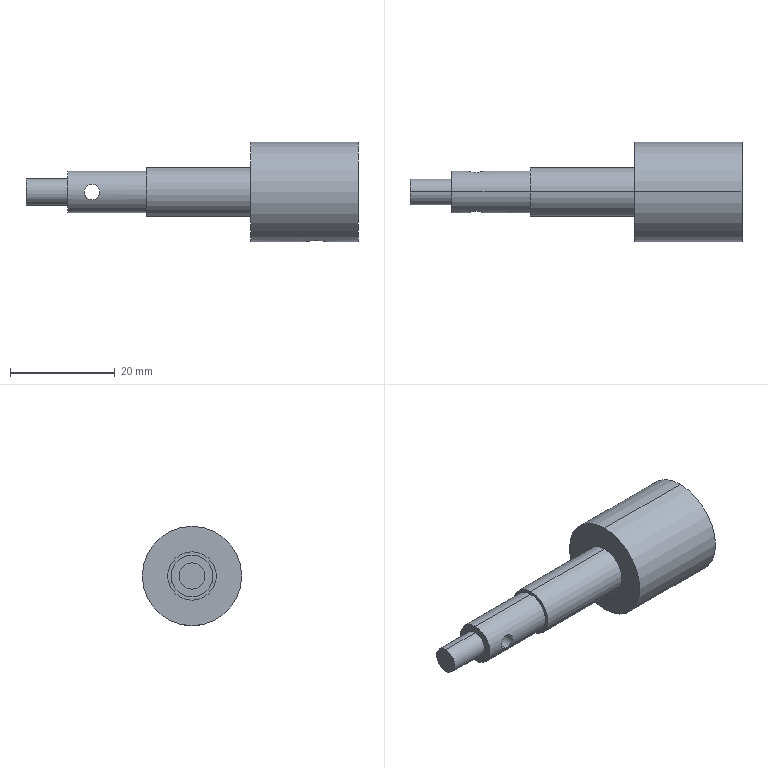Part | SolidWorks | features BaseBody 1 | 1 solid | 20 faces | box 63.5 x 19 x 19 mm | volume 6544 mm3 | cylinder 14 | plane 6 | commonest cylinder face diameters 3 x2 4 x2 5 x2 8 x2 9.26 x2 10 x2
STEP:
#1=CARTESIAN_POINT('',(-19.873,0.,-9.5));
#2=VERTEX_POINT('',#1);
#3=CARTESIAN_POINT('',(-15.873,0.,-9.5));
#4=VERTEX_POINT('',#3);
#5=CARTESIAN_POINT('',(-19.873,0.,-9.5));
#6=CARTESIAN_POINT('',(-19.873,-0.2614,-9.5));
#7=CARTESIAN_POINT('',(-19.82,-0.5253,-9.489));
#8=CARTESIAN_POINT('',(-19.67,-0.8864,-9.459));
#9=CARTESIAN_POINT('',(-19.608,-1.003,-9.448));
#10=CARTESIAN_POINT('',(-19.462,-1.221,-9.422));
#11=CARTESIAN_POINT('',(-19.38,-1.321,-9.408));
#12=CARTESIAN_POINT('',(-19.196,-1.506,-9.38));
#13=CARTESIAN_POINT('',(-19.093,-1.59,-9.366));
#14=CARTESIAN_POINT('',(-18.877,-1.735,-9.341));
#15=CARTESIAN_POINT('',(-18.762,-1.796,-9.329));
#16=CARTESIAN_POINT('',(-18.398,-1.948,-9.299));
#17=CARTESIAN_POINT('',(-18.138,-2.,-9.287));
#18=CARTESIAN_POINT('',(-17.742,-2.,-9.287));
#19=CARTESIAN_POINT('',(-17.612,-1.987,-9.29));
#20=CARTESIAN_POINT('',(-17.355,-1.936,-9.301));
#21=CARTESIAN_POINT('',(-17.228,-1.898,-9.309));
#22=CARTESIAN_POINT('',(-16.986,-1.797,-9.329));
#23=CARTESIAN_POINT('',(-16.871,-1.736,-9.34));
#24=CARTESIAN_POINT('',(-16.653,-1.591,-9.366));
#25=CARTESIAN_POINT('',(-16.551,-1.507,-9.38));
#26=CARTESIAN_POINT('',(-16.276,-1.231,-9.422));
#27=CARTESIAN_POINT('',(-16.126,-1.009,-9.449));
#28=CARTESIAN_POINT('',(-15.976,-0.6483,-9.479));
#29=CARTESIAN_POINT('',(-15.937,-0.5213,-9.487));
#30=CARTESIAN_POINT('',(-15.886,-0.2633,-9.497));
#31=CARTESIAN_POINT('',(-15.873,-0.1325,-9.5));
#32=CARTESIAN_POINT('',(-15.873,0.,-9.5));
#33=B_SPLINE_CURVE_WITH_KNOTS('',3,(#5,#6,#7,#8,#9,#10,#11,#12,#13,#14,#15,#16,#17,#18,#19,#20,#21,#22,#23,#24,#25,#26,#27,#28,#29,#30,#31,#32),.UNSPECIFIED.,.F.,.F.,(4,2,2,2,2,2,2,2,2,2,2,2,2,4),(0.00627,0.007054,0.007446,0.007838,0.00823,0.008621,0.009405,0.009797,0.01019,0.01058,0.01097,0.01176,0.01215,0.01254),.UNSPECIFIED.);
#34=EDGE_CURVE('',#2,#4,#33,.T.);
#35=ORIENTED_EDGE('',*,*,#34,.F.);
#36=CARTESIAN_POINT('',(-19.873,0.,-5.));
#37=VERTEX_POINT('',#36);
#38=CARTESIAN_POINT('',(-19.873,0.,-17.5));
#39=DIRECTION('',(0.,0.,1.));
#40=VECTOR('',#39,1000.);
#41=LINE('',#38,#40);
#42=EDGE_CURVE('',#2,#37,#41,.T.);
#43=ORIENTED_EDGE('',*,*,#42,.T.);
#44=CARTESIAN_POINT('',(-15.873,0.,-5.));
#45=VERTEX_POINT('',#44);
#46=CARTESIAN_POINT('',(-15.873,0.,-5.));
#47=CARTESIAN_POINT('',(-15.873,-0.1316,-5.));
#48=CARTESIAN_POINT('',(-15.886,-0.2649,-4.995));
#49=CARTESIAN_POINT('',(-15.938,-0.5241,-4.974));
#50=CARTESIAN_POINT('',(-15.976,-0.6493,-4.959));
#51=CARTESIAN_POINT('',(-16.077,-0.8912,-4.921));
#52=CARTESIAN_POINT('',(-16.14,-1.008,-4.899));
#53=CARTESIAN_POINT('',(-16.285,-1.223,-4.849));
#54=CARTESIAN_POINT('',(-16.367,-1.323,-4.823));
#55=CARTESIAN_POINT('',(-16.552,-1.507,-4.768));
#56=CARTESIAN_POINT('',(-16.652,-1.589,-4.741));
#57=CARTESIAN_POINT('',(-16.866,-1.733,-4.691));
#58=CARTESIAN_POINT('',(-16.983,-1.796,-4.667));
#59=CARTESIAN_POINT('',(-17.224,-1.896,-4.627));
#60=CARTESIAN_POINT('',(-17.349,-1.935,-4.611));
#61=CARTESIAN_POINT('',(-17.607,-1.987,-4.589));
#62=CARTESIAN_POINT('',(-17.741,-2.,-4.583));
#63=CARTESIAN_POINT('',(-18.136,-2.,-4.583));
#64=CARTESIAN_POINT('',(-18.401,-1.946,-4.607));
#65=CARTESIAN_POINT('',(-18.763,-1.796,-4.667));
#66=CARTESIAN_POINT('',(-18.879,-1.733,-4.691));
#67=CARTESIAN_POINT('',(-19.095,-1.589,-4.742));
#68=CARTESIAN_POINT('',(-19.194,-1.507,-4.769));
#69=CARTESIAN_POINT('',(-19.378,-1.323,-4.823));
#70=CARTESIAN_POINT('',(-19.461,-1.222,-4.85));
#71=CARTESIAN_POINT('',(-19.606,-1.007,-4.899));
#72=CARTESIAN_POINT('',(-19.667,-0.8926,-4.921));
#73=CARTESIAN_POINT('',(-19.82,-0.5273,-4.978));
#74=CARTESIAN_POINT('',(-19.873,-0.2671,-5.));
#75=CARTESIAN_POINT('',(-19.873,0.,-5.));
#76=B_SPLINE_CURVE_WITH_KNOTS('',3,(#46,#47,#48,#49,#50,#51,#52,#53,#54,#55,#56,#57,#58,#59,#60,#61,#62,#63,#64,#65,#66,#67,#68,#69,#70,#71,#72,#73,#74,#75),.UNSPECIFIED.,.F.,.F.,(4,2,2,2,2,2,2,2,2,2,2,2,2,2,4),(0.00632,0.006715,0.007109,0.007504,0.007899,0.008293,0.008688,0.009083,0.009478,0.01027,0.01066,0.01106,0.01145,0.01185,0.01264),.UNSPECIFIED.);
#77=EDGE_CURVE('',#45,#37,#76,.T.);
#78=ORIENTED_EDGE('',*,*,#77,.F.);
#79=CARTESIAN_POINT('',(-15.873,0.,-17.5));
#80=DIRECTION('',(0.,0.,1.));
#81=VECTOR('',#80,1000.);
#82=LINE('',#79,#81);
#83=EDGE_CURVE('',#4,#45,#82,.T.);
#84=ORIENTED_EDGE('',*,*,#83,.F.);
#85=EDGE_LOOP('',(#35,#43,#78,#84));
#86=FACE_OUTER_BOUND('',#85,.T.);
#87=CARTESIAN_POINT('',(-17.873,0.,-17.5));
#88=DIRECTION('',(0.,0.,1.));
#89=DIRECTION('',(1.,0.,0.));
#90=AXIS2_PLACEMENT_3D('',#87,#88,#89);
#91=CYLINDRICAL_SURFACE('',#90,2.);
#92=ADVANCED_FACE('',(#86),#91,.F.);
#93=CARTESIAN_POINT('',(-60.756,-3.708,-1.5));
#94=VERTEX_POINT('',#93);
#95=CARTESIAN_POINT('',(-60.756,-3.708,1.5));
#96=VERTEX_POINT('',#95);
#97=CARTESIAN_POINT('',(-60.756,-3.708,-1.5));
#98=CARTESIAN_POINT('',(-60.953,-3.708,-1.5));
#99=CARTESIAN_POINT('',(-61.152,-3.725,-1.46));
#100=CARTESIAN_POINT('',(-61.424,-3.767,-1.347));
#101=CARTESIAN_POINT('',(-61.511,-3.783,-1.3));
#102=CARTESIAN_POINT('',(-61.672,-3.819,-1.191));
#103=CARTESIAN_POINT('',(-61.747,-3.838,-1.13));
#104=CARTESIAN_POINT('',(-61.956,-3.895,-0.9215));
#105=CARTESIAN_POINT('',(-62.065,-3.932,-0.7581));
#106=CARTESIAN_POINT('',(-62.179,-3.971,-0.4854));
#107=CARTESIAN_POINT('',(-62.207,-3.982,-0.3917));
#108=CARTESIAN_POINT('',(-62.246,-3.996,-0.1986));
#109=CARTESIAN_POINT('',(-62.256,-4.,-0.09814));
#110=CARTESIAN_POINT('',(-62.256,-4.,0.1984));
#111=CARTESIAN_POINT('',(-62.216,-3.984,0.3972));
#112=CARTESIAN_POINT('',(-62.065,-3.932,0.7586));
#113=CARTESIAN_POINT('',(-61.953,-3.894,0.924));
#114=CARTESIAN_POINT('',(-61.747,-3.838,1.13));
#115=CARTESIAN_POINT('',(-61.67,-3.818,1.193));
#116=CARTESIAN_POINT('',(-61.509,-3.783,1.301));
#117=CARTESIAN_POINT('',(-61.423,-3.767,1.347));
#118=CARTESIAN_POINT('',(-61.15,-3.725,1.461));
#119=CARTESIAN_POINT('',(-60.956,-3.708,1.5));
#120=CARTESIAN_POINT('',(-60.756,-3.708,1.5));
#121=B_SPLINE_CURVE_WITH_KNOTS('',3,(#97,#98,#99,#100,#101,#102,#103,#104,#105,#106,#107,#108,#109,#110,#111,#112,#113,#114,#115,#116,#117,#118,#119,#120),.UNSPECIFIED.,.F.,.F.,(4,2,2,2,2,2,2,2,2,2,2,4),(0.004733,0.005325,0.00562,0.005916,0.006508,0.006803,0.007099,0.007691,0.008282,0.008578,0.008874,0.009465),.UNSPECIFIED.);
#122=EDGE_CURVE('',#94,#96,#121,.T.);
#123=ORIENTED_EDGE('',*,*,#122,.F.);
#124=CARTESIAN_POINT('',(-60.756,3.708,-1.5));
#125=VERTEX_POINT('',#124);
#126=CARTESIAN_POINT('',(-60.756,-8.75,-1.5));
#127=DIRECTION('',(0.,1.,0.));
#128=VECTOR('',#127,1000.);
#129=LINE('',#126,#128);
#130=EDGE_CURVE('',#94,#125,#129,.T.);
#131=ORIENTED_EDGE('',*,*,#130,.T.);
#132=CARTESIAN_POINT('',(-60.756,3.708,1.5));
#133=VERTEX_POINT('',#132);
#134=CARTESIAN_POINT('',(-60.756,3.708,1.5));
#135=CARTESIAN_POINT('',(-60.856,3.708,1.5));
#136=CARTESIAN_POINT('',(-60.954,3.712,1.49));
#137=CARTESIAN_POINT('',(-61.147,3.727,1.451));
#138=CARTESIAN_POINT('',(-61.243,3.739,1.422));
#139=CARTESIAN_POINT('',(-61.515,3.781,1.309));
#140=CARTESIAN_POINT('',(-61.68,3.819,1.198));
#141=CARTESIAN_POINT('',(-61.954,3.895,0.9235));
#142=CARTESIAN_POINT('',(-62.065,3.932,0.7577));
#143=CARTESIAN_POINT('',(-62.178,3.971,0.4873));
#144=CARTESIAN_POINT('',(-62.207,3.982,0.3918));
#145=CARTESIAN_POINT('',(-62.246,3.996,0.1976));
#146=CARTESIAN_POINT('',(-62.256,4.,0.09965));
#147=CARTESIAN_POINT('',(-62.256,4.,-0.09818));
#148=CARTESIAN_POINT('',(-62.246,3.996,-0.1986));
#149=CARTESIAN_POINT('',(-62.207,3.982,-0.3918));
#150=CARTESIAN_POINT('',(-62.178,3.971,-0.4859));
#151=CARTESIAN_POINT('',(-62.102,3.945,-0.6688));
#152=CARTESIAN_POINT('',(-62.056,3.929,-0.7549));
#153=CARTESIAN_POINT('',(-61.947,3.894,-0.9165));
#154=CARTESIAN_POINT('',(-61.884,3.875,-0.9928));
#155=CARTESIAN_POINT('',(-61.747,3.838,-1.13));
#156=CARTESIAN_POINT('',(-61.672,3.819,-1.192));
#157=CARTESIAN_POINT('',(-61.51,3.783,-1.3));
#158=CARTESIAN_POINT('',(-61.422,3.766,-1.347));
#159=CARTESIAN_POINT('',(-61.152,3.725,-1.46));
#160=CARTESIAN_POINT('',(-60.953,3.708,-1.5));
#161=CARTESIAN_POINT('',(-60.756,3.708,-1.5));
#162=B_SPLINE_CURVE_WITH_KNOTS('',3,(#134,#135,#136,#137,#138,#139,#140,#141,#142,#143,#144,#145,#146,#147,#148,#149,#150,#151,#152,#153,#154,#155,#156,#157,#158,#159,#160,#161),.UNSPECIFIED.,.F.,.F.,(4,2,2,2,2,2,2,2,2,2,2,2,2,4),(0.,0.0002958,0.0005916,0.001183,0.001775,0.002071,0.002367,0.002662,0.002958,0.003254,0.00355,0.003846,0.004142,0.004733),.UNSPECIFIED.);
#163=EDGE_CURVE('',#133,#125,#162,.T.);
#164=ORIENTED_EDGE('',*,*,#163,.F.);
#165=CARTESIAN_POINT('',(-60.756,-8.75,1.5));
#166=DIRECTION('',(0.,1.,0.));
#167=VECTOR('',#166,1000.);
#168=LINE('',#165,#167);
#169=EDGE_CURVE('',#96,#133,#168,.T.);
#170=ORIENTED_EDGE('',*,*,#169,.F.);
#171=EDGE_LOOP('',(#123,#131,#164,#170));
#172=FACE_OUTER_BOUND('',#171,.T.);
#173=CARTESIAN_POINT('',(-60.756,-8.75,0.));
#174=DIRECTION('',(0.,1.,0.));
#175=DIRECTION('',(0.,0.,1.));
#176=AXIS2_PLACEMENT_3D('',#173,#174,#175);
#177=CYLINDRICAL_SURFACE('',#176,1.5);
#178=ADVANCED_FACE('',(#172),#177,.F.);
#179=CARTESIAN_POINT('',(-27.873,0.,5.));
#180=VERTEX_POINT('',#179);
#181=CARTESIAN_POINT('',(-27.873,0.,-5.));
#182=VERTEX_POINT('',#181);
#183=CARTESIAN_POINT('',(-27.873,0.,0.));
#184=DIRECTION('',(1.,0.,0.));
#185=DIRECTION('',(0.,0.,-1.));
#186=AXIS2_PLACEMENT_3D('',#183,#184,#185);
#187=CIRCLE('',#186,5.);
#188=EDGE_CURVE('',#180,#182,#187,.T.);
#189=ORIENTED_EDGE('',*,*,#188,.F.);
#190=CARTESIAN_POINT('',(-9.873,0.,5.));
#191=VERTEX_POINT('',#190);
#192=CARTESIAN_POINT('',(-27.873,0.,5.));
#193=DIRECTION('',(1.,0.,0.));
#194=VECTOR('',#193,1000.);
#195=LINE('',#192,#194);
#196=EDGE_CURVE('',#180,#191,#195,.T.);
#197=ORIENTED_EDGE('',*,*,#196,.T.);
#198=CARTESIAN_POINT('',(-9.873,0.,-5.));
#199=VERTEX_POINT('',#198);
#200=CARTESIAN_POINT('',(-9.873,0.,0.));
#201=DIRECTION('',(1.,0.,0.));
#202=DIRECTION('',(0.,0.,-1.));
#203=AXIS2_PLACEMENT_3D('',#200,#201,#202);
#204=CIRCLE('',#203,5.);
#205=EDGE_CURVE('',#191,#199,#204,.T.);
#206=ORIENTED_EDGE('',*,*,#205,.T.);
#207=CARTESIAN_POINT('',(-27.873,0.,-5.));
#208=DIRECTION('',(1.,0.,0.));
#209=VECTOR('',#208,1000.);
#210=LINE('',#207,#209);
#211=EDGE_CURVE('',#45,#199,#210,.T.);
#212=ORIENTED_EDGE('',*,*,#211,.F.);
#213=ORIENTED_EDGE('',*,*,#77,.T.);
#214=CARTESIAN_POINT('',(-27.873,0.,-5.));
#215=DIRECTION('',(1.,0.,0.));
#216=VECTOR('',#215,1000.);
#217=LINE('',#214,#216);
#218=EDGE_CURVE('',#182,#37,#217,.T.);
#219=ORIENTED_EDGE('',*,*,#218,.F.);
#220=EDGE_LOOP('',(#189,#197,#206,#212,#213,#219));
#221=FACE_OUTER_BOUND('',#220,.T.);
#222=CARTESIAN_POINT('',(-27.873,0.,0.));
#223=DIRECTION('',(1.,0.,0.));
#224=DIRECTION('',(0.,0.,-1.));
#225=AXIS2_PLACEMENT_3D('',#222,#223,#224);
#226=CYLINDRICAL_SURFACE('',#225,5.);
#227=ADVANCED_FACE('',(#221),#226,.F.);
#228=CARTESIAN_POINT('',(-9.873,0.,9.5));
#229=VERTEX_POINT('',#228);
#230=CARTESIAN_POINT('',(-9.873,0.,-9.5));
#231=VERTEX_POINT('',#230);
#232=CARTESIAN_POINT('',(-9.873,0.,0.));
#233=DIRECTION('',(-1.,0.,0.));
#234=DIRECTION('',(0.,0.,1.));
#235=AXIS2_PLACEMENT_3D('',#232,#233,#234);
#236=CIRCLE('',#235,9.5);
#237=EDGE_CURVE('',#229,#231,#236,.T.);
#238=ORIENTED_EDGE('',*,*,#237,.T.);
#239=CARTESIAN_POINT('',(-48.597,0.,-9.5));
#240=DIRECTION('',(-1.,0.,0.));
#241=VECTOR('',#240,1000.);
#242=LINE('',#239,#241);
#243=EDGE_CURVE('',#231,#4,#242,.T.);
#244=ORIENTED_EDGE('',*,*,#243,.T.);
#245=CARTESIAN_POINT('',(-15.873,0.,-9.5));
#246=CARTESIAN_POINT('',(-15.873,0.1325,-9.5));
#247=CARTESIAN_POINT('',(-15.886,0.2628,-9.497));
#248=CARTESIAN_POINT('',(-15.937,0.5189,-9.487));
#249=CARTESIAN_POINT('',(-15.975,0.6462,-9.479));
#250=CARTESIAN_POINT('',(-16.076,0.8882,-9.459));
#251=CARTESIAN_POINT('',(-16.137,1.003,-9.448));
#252=CARTESIAN_POINT('',(-16.283,1.22,-9.422));
#253=CARTESIAN_POINT('',(-16.367,1.323,-9.408));
#254=CARTESIAN_POINT('',(-16.643,1.598,-9.366));
#255=CARTESIAN_POINT('',(-16.865,1.747,-9.338));
#256=CARTESIAN_POINT('',(-17.346,1.947,-9.299));
#257=CARTESIAN_POINT('',(-17.61,2.,-9.287));
#258=CARTESIAN_POINT('',(-18.003,2.,-9.287));
#259=CARTESIAN_POINT('',(-18.136,1.987,-9.29));
#260=CARTESIAN_POINT('',(-18.393,1.936,-9.301));
#261=CARTESIAN_POINT('',(-18.517,1.898,-9.309));
#262=CARTESIAN_POINT('',(-18.881,1.747,-9.339));
#263=CARTESIAN_POINT('',(-19.101,1.6,-9.366));
#264=CARTESIAN_POINT('',(-19.38,1.321,-9.408));
#265=CARTESIAN_POINT('',(-19.462,1.221,-9.422));
#266=CARTESIAN_POINT('',(-19.607,1.004,-9.447));
#267=CARTESIAN_POINT('',(-19.67,0.8871,-9.459));
#268=CARTESIAN_POINT('',(-19.77,0.6454,-9.479));
#269=CARTESIAN_POINT('',(-19.808,0.5207,-9.487));
#270=CARTESIAN_POINT('',(-19.86,0.2635,-9.497));
#271=CARTESIAN_POINT('',(-19.873,0.1307,-9.5));
#272=CARTESIAN_POINT('',(-19.873,0.,-9.5));
#273=B_SPLINE_CURVE_WITH_KNOTS('',3,(#245,#246,#247,#248,#249,#250,#251,#252,#253,#254,#255,#256,#257,#258,#259,#260,#261,#262,#263,#264,#265,#266,#267,#268,#269,#270,#271,#272),.UNSPECIFIED.,.F.,.F.,(4,2,2,2,2,2,2,2,2,2,2,2,2,4),(0.,0.0003919,0.0007838,0.001176,0.001568,0.002351,0.003135,0.003527,0.003919,0.004703,0.005095,0.005487,0.005879,0.00627),.UNSPECIFIED.);
#274=EDGE_CURVE('',#4,#2,#273,.T.);
#275=ORIENTED_EDGE('',*,*,#274,.T.);
#276=CARTESIAN_POINT('',(-30.373,0.,-9.5));
#277=VERTEX_POINT('',#276);
#278=CARTESIAN_POINT('',(-48.597,0.,-9.5));
#279=DIRECTION('',(-1.,0.,0.));
#280=VECTOR('',#279,1000.);
#281=LINE('',#278,#280);
#282=EDGE_CURVE('',#2,#277,#281,.T.);
#283=ORIENTED_EDGE('',*,*,#282,.T.);
#284=CARTESIAN_POINT('',(-30.373,0.,9.5));
#285=VERTEX_POINT('',#284);
#286=CARTESIAN_POINT('',(-30.373,0.,0.));
#287=DIRECTION('',(-1.,0.,0.));
#288=DIRECTION('',(0.,0.,1.));
#289=AXIS2_PLACEMENT_3D('',#286,#287,#288);
#290=CIRCLE('',#289,9.5);
#291=EDGE_CURVE('',#285,#277,#290,.T.);
#292=ORIENTED_EDGE('',*,*,#291,.F.);
#293=CARTESIAN_POINT('',(-48.597,0.,9.5));
#294=DIRECTION('',(-1.,0.,0.));
#295=VECTOR('',#294,1000.);
#296=LINE('',#293,#295);
#297=EDGE_CURVE('',#229,#285,#296,.T.);
#298=ORIENTED_EDGE('',*,*,#297,.F.);
#299=EDGE_LOOP('',(#238,#244,#275,#283,#292,#298));
#300=FACE_OUTER_BOUND('',#299,.T.);
#301=CARTESIAN_POINT('',(-48.597,0.,0.));
#302=DIRECTION('',(-1.,0.,0.));
#303=DIRECTION('',(0.,0.,1.));
#304=AXIS2_PLACEMENT_3D('',#301,#302,#303);
#305=CYLINDRICAL_SURFACE('',#304,9.5);
#306=ADVANCED_FACE('',(#300),#305,.T.);
#307=CARTESIAN_POINT('',(-30.373,0.,4.63));
#308=VERTEX_POINT('',#307);
#309=CARTESIAN_POINT('',(-30.373,0.,-4.63));
#310=VERTEX_POINT('',#309);
#311=CARTESIAN_POINT('',(-30.373,0.,0.));
#312=DIRECTION('',(-1.,0.,0.));
#313=DIRECTION('',(0.,0.,1.));
#314=AXIS2_PLACEMENT_3D('',#311,#312,#313);
#315=CIRCLE('',#314,4.63);
#316=EDGE_CURVE('',#308,#310,#315,.T.);
#317=ORIENTED_EDGE('',*,*,#316,.T.);
#318=CARTESIAN_POINT('',(-50.373,0.,-4.63));
#319=VERTEX_POINT('',#318);
#320=CARTESIAN_POINT('',(-48.597,0.,-4.63));
#321=DIRECTION('',(-1.,0.,0.));
#322=VECTOR('',#321,1000.);
#323=LINE('',#320,#322);
#324=EDGE_CURVE('',#310,#319,#323,.T.);
#325=ORIENTED_EDGE('',*,*,#324,.T.);
#326=CARTESIAN_POINT('',(-50.373,0.,4.63));
#327=VERTEX_POINT('',#326);
#328=CARTESIAN_POINT('',(-50.373,0.,0.));
#329=DIRECTION('',(-1.,0.,0.));
#330=DIRECTION('',(0.,0.,1.));
#331=AXIS2_PLACEMENT_3D('',#328,#329,#330);
#332=CIRCLE('',#331,4.63);
#333=EDGE_CURVE('',#327,#319,#332,.T.);
#334=ORIENTED_EDGE('',*,*,#333,.F.);
#335=CARTESIAN_POINT('',(-48.597,0.,4.63));
#336=DIRECTION('',(-1.,0.,0.));
#337=VECTOR('',#336,1000.);
#338=LINE('',#335,#337);
#339=EDGE_CURVE('',#308,#327,#338,.T.);
#340=ORIENTED_EDGE('',*,*,#339,.F.);
#341=EDGE_LOOP('',(#317,#325,#334,#340));
#342=FACE_OUTER_BOUND('',#341,.T.);
#343=CARTESIAN_POINT('',(-48.597,0.,0.));
#344=DIRECTION('',(-1.,0.,0.));
#345=DIRECTION('',(0.,0.,1.));
#346=AXIS2_PLACEMENT_3D('',#343,#344,#345);
#347=CYLINDRICAL_SURFACE('',#346,4.63);
#348=ADVANCED_FACE('',(#342),#347,.T.);
#349=ORIENTED_EDGE('',*,*,#163,.T.);
#350=CARTESIAN_POINT('',(-60.756,3.708,-1.5));
#351=CARTESIAN_POINT('',(-60.559,3.708,-1.5));
#352=CARTESIAN_POINT('',(-60.36,3.725,-1.46));
#353=CARTESIAN_POINT('',(-60.088,3.767,-1.347));
#354=CARTESIAN_POINT('',(-60.001,3.783,-1.3));
#355=CARTESIAN_POINT('',(-59.839,3.819,-1.191));
#356=CARTESIAN_POINT('',(-59.764,3.838,-1.13));
#357=CARTESIAN_POINT('',(-59.556,3.895,-0.9215));
#358=CARTESIAN_POINT('',(-59.447,3.932,-0.7581));
#359=CARTESIAN_POINT('',(-59.333,3.971,-0.4854));
#360=CARTESIAN_POINT('',(-59.305,3.982,-0.3917));
#361=CARTESIAN_POINT('',(-59.266,3.996,-0.1986));
#362=CARTESIAN_POINT('',(-59.256,4.,-0.09814));
#363=CARTESIAN_POINT('',(-59.256,4.,0.1984));
#364=CARTESIAN_POINT('',(-59.296,3.984,0.3972));
#365=CARTESIAN_POINT('',(-59.447,3.932,0.7586));
#366=CARTESIAN_POINT('',(-59.558,3.894,0.924));
#367=CARTESIAN_POINT('',(-59.765,3.838,1.13));
#368=CARTESIAN_POINT('',(-59.841,3.818,1.193));
#369=CARTESIAN_POINT('',(-60.003,3.783,1.301));
#370=CARTESIAN_POINT('',(-60.088,3.767,1.347));
#371=CARTESIAN_POINT('',(-60.361,3.725,1.461));
#372=CARTESIAN_POINT('',(-60.556,3.708,1.5));
#373=CARTESIAN_POINT('',(-60.756,3.708,1.5));
#374=B_SPLINE_CURVE_WITH_KNOTS('',3,(#350,#351,#352,#353,#354,#355,#356,#357,#358,#359,#360,#361,#362,#363,#364,#365,#366,#367,#368,#369,#370,#371,#372,#373),.UNSPECIFIED.,.F.,.F.,(4,2,2,2,2,2,2,2,2,2,2,4),(0.004733,0.005325,0.00562,0.005916,0.006508,0.006803,0.007099,0.007691,0.008282,0.008578,0.008874,0.009465),.UNSPECIFIED.);
#375=EDGE_CURVE('',#125,#133,#374,.T.);
#376=ORIENTED_EDGE('',*,*,#375,.T.);
#377=EDGE_LOOP('',(#349,#376));
#378=FACE_BOUND('',#377,.T.);
#379=CARTESIAN_POINT('',(-50.373,0.,4.));
#380=VERTEX_POINT('',#379);
#381=CARTESIAN_POINT('',(-50.373,0.,-4.));
#382=VERTEX_POINT('',#381);
#383=CARTESIAN_POINT('',(-50.373,0.,0.));
#384=DIRECTION('',(-1.,0.,0.));
#385=DIRECTION('',(0.,0.,1.));
#386=AXIS2_PLACEMENT_3D('',#383,#384,#385);
#387=CIRCLE('',#386,4.);
#388=EDGE_CURVE('',#380,#382,#387,.T.);
#389=ORIENTED_EDGE('',*,*,#388,.T.);
#390=CARTESIAN_POINT('',(-65.373,0.,-4.));
#391=VERTEX_POINT('',#390);
#392=CARTESIAN_POINT('',(-48.597,0.,-4.));
#393=DIRECTION('',(-1.,0.,0.));
#394=VECTOR('',#393,1000.);
#395=LINE('',#392,#394);
#396=EDGE_CURVE('',#382,#391,#395,.T.);
#397=ORIENTED_EDGE('',*,*,#396,.T.);
#398=CARTESIAN_POINT('',(-65.373,0.,4.));
#399=VERTEX_POINT('',#398);
#400=CARTESIAN_POINT('',(-65.373,0.,0.));
#401=DIRECTION('',(-1.,0.,0.));
#402=DIRECTION('',(0.,0.,1.));
#403=AXIS2_PLACEMENT_3D('',#400,#401,#402);
#404=CIRCLE('',#403,4.);
#405=EDGE_CURVE('',#399,#391,#404,.T.);
#406=ORIENTED_EDGE('',*,*,#405,.F.);
#407=CARTESIAN_POINT('',(-48.597,0.,4.));
#408=DIRECTION('',(-1.,0.,0.));
#409=VECTOR('',#408,1000.);
#410=LINE('',#407,#409);
#411=EDGE_CURVE('',#380,#399,#410,.T.);
#412=ORIENTED_EDGE('',*,*,#411,.F.);
#413=EDGE_LOOP('',(#389,#397,#406,#412));
#414=FACE_OUTER_BOUND('',#413,.T.);
#415=CARTESIAN_POINT('',(-48.597,0.,0.));
#416=DIRECTION('',(-1.,0.,0.));
#417=DIRECTION('',(0.,0.,1.));
#418=AXIS2_PLACEMENT_3D('',#415,#416,#417);
#419=CYLINDRICAL_SURFACE('',#418,4.);
#420=ADVANCED_FACE('',(#378,#414),#419,.T.);
#421=CARTESIAN_POINT('',(-65.373,0.,2.5));
#422=VERTEX_POINT('',#421);
#423=CARTESIAN_POINT('',(-65.373,0.,-2.5));
#424=VERTEX_POINT('',#423);
#425=CARTESIAN_POINT('',(-65.373,0.,0.));
#426=DIRECTION('',(-1.,0.,0.));
#427=DIRECTION('',(0.,0.,1.));
#428=AXIS2_PLACEMENT_3D('',#425,#426,#427);
#429=CIRCLE('',#428,2.5);
#430=EDGE_CURVE('',#422,#424,#429,.T.);
#431=ORIENTED_EDGE('',*,*,#430,.T.);
#432=CARTESIAN_POINT('',(-73.373,0.,-2.5));
#433=VERTEX_POINT('',#432);
#434=CARTESIAN_POINT('',(-48.597,0.,-2.5));
#435=DIRECTION('',(-1.,0.,0.));
#436=VECTOR('',#435,1000.);
#437=LINE('',#434,#436);
#438=EDGE_CURVE('',#424,#433,#437,.T.);
#439=ORIENTED_EDGE('',*,*,#438,.T.);
#440=CARTESIAN_POINT('',(-73.373,0.,2.5));
#441=VERTEX_POINT('',#440);
#442=CARTESIAN_POINT('',(-73.373,0.,0.));
#443=DIRECTION('',(-1.,0.,0.));
#444=DIRECTION('',(0.,0.,1.));
#445=AXIS2_PLACEMENT_3D('',#442,#443,#444);
#446=CIRCLE('',#445,2.5);
#447=EDGE_CURVE('',#441,#433,#446,.T.);
#448=ORIENTED_EDGE('',*,*,#447,.F.);
#449=CARTESIAN_POINT('',(-48.597,0.,2.5));
#450=DIRECTION('',(-1.,0.,0.));
#451=VECTOR('',#450,1000.);
#452=LINE('',#449,#451);
#453=EDGE_CURVE('',#422,#441,#452,.T.);
#454=ORIENTED_EDGE('',*,*,#453,.F.);
#455=EDGE_LOOP('',(#431,#439,#448,#454));
#456=FACE_OUTER_BOUND('',#455,.T.);
#457=CARTESIAN_POINT('',(-48.597,0.,0.));
#458=DIRECTION('',(-1.,0.,0.));
#459=DIRECTION('',(0.,0.,1.));
#460=AXIS2_PLACEMENT_3D('',#457,#458,#459);
#461=CYLINDRICAL_SURFACE('',#460,2.5);
#462=ADVANCED_FACE('',(#456),#461,.T.);
#463=ORIENTED_EDGE('',*,*,#447,.T.);
#464=CARTESIAN_POINT('',(-73.373,0.,0.));
#465=DIRECTION('',(-1.,0.,0.));
#466=DIRECTION('',(0.,0.,1.));
#467=AXIS2_PLACEMENT_3D('',#464,#465,#466);
#468=CIRCLE('',#467,2.5);
#469=EDGE_CURVE('',#433,#441,#468,.T.);
#470=ORIENTED_EDGE('',*,*,#469,.T.);
#471=EDGE_LOOP('',(#463,#470));
#472=FACE_OUTER_BOUND('',#471,.T.);
#473=CARTESIAN_POINT('',(-73.373,0.,0.));
#474=DIRECTION('',(1.,0.,0.));
#475=DIRECTION('',(0.,0.,-1.));
#476=AXIS2_PLACEMENT_3D('',#473,#474,#475);
#477=PLANE('',#476);
#478=ADVANCED_FACE('',(#472),#477,.F.);
#479=ORIENTED_EDGE('',*,*,#438,.F.);
#480=CARTESIAN_POINT('',(-65.373,0.,0.));
#481=DIRECTION('',(-1.,0.,0.));
#482=DIRECTION('',(0.,0.,1.));
#483=AXIS2_PLACEMENT_3D('',#480,#481,#482);
#484=CIRCLE('',#483,2.5);
#485=EDGE_CURVE('',#424,#422,#484,.T.);
#486=ORIENTED_EDGE('',*,*,#485,.T.);
#487=ORIENTED_EDGE('',*,*,#453,.T.);
#488=ORIENTED_EDGE('',*,*,#469,.F.);
#489=EDGE_LOOP('',(#479,#486,#487,#488));
#490=FACE_OUTER_BOUND('',#489,.T.);
#491=CARTESIAN_POINT('',(-48.597,0.,0.));
#492=DIRECTION('',(-1.,0.,0.));
#493=DIRECTION('',(0.,0.,1.));
#494=AXIS2_PLACEMENT_3D('',#491,#492,#493);
#495=CYLINDRICAL_SURFACE('',#494,2.5);
#496=ADVANCED_FACE('',(#490),#495,.T.);
#497=ORIENTED_EDGE('',*,*,#430,.F.);
#498=ORIENTED_EDGE('',*,*,#485,.F.);
#499=EDGE_LOOP('',(#497,#498));
#500=FACE_BOUND('',#499,.T.);
#501=ORIENTED_EDGE('',*,*,#405,.T.);
#502=CARTESIAN_POINT('',(-65.373,0.,0.));
#503=DIRECTION('',(-1.,0.,0.));
#504=DIRECTION('',(0.,0.,1.));
#505=AXIS2_PLACEMENT_3D('',#502,#503,#504);
#506=CIRCLE('',#505,4.);
#507=EDGE_CURVE('',#391,#399,#506,.T.);
#508=ORIENTED_EDGE('',*,*,#507,.T.);
#509=EDGE_LOOP('',(#501,#508));
#510=FACE_OUTER_BOUND('',#509,.T.);
#511=CARTESIAN_POINT('',(-65.373,0.,-2.5));
#512=DIRECTION('',(1.,0.,0.));
#513=DIRECTION('',(0.,0.,-1.));
#514=AXIS2_PLACEMENT_3D('',#511,#512,#513);
#515=PLANE('',#514);
#516=ADVANCED_FACE('',(#500,#510),#515,.F.);
#517=ORIENTED_EDGE('',*,*,#396,.F.);
#518=CARTESIAN_POINT('',(-50.373,0.,0.));
#519=DIRECTION('',(-1.,0.,0.));
#520=DIRECTION('',(0.,0.,1.));
#521=AXIS2_PLACEMENT_3D('',#518,#519,#520);
#522=CIRCLE('',#521,4.);
#523=EDGE_CURVE('',#382,#380,#522,.T.);
#524=ORIENTED_EDGE('',*,*,#523,.T.);
#525=ORIENTED_EDGE('',*,*,#411,.T.);
#526=ORIENTED_EDGE('',*,*,#507,.F.);
#527=EDGE_LOOP('',(#517,#524,#525,#526));
#528=FACE_OUTER_BOUND('',#527,.T.);
#529=CARTESIAN_POINT('',(-60.756,-3.708,1.5));
#530=CARTESIAN_POINT('',(-60.656,-3.708,1.5));
#531=CARTESIAN_POINT('',(-60.558,-3.712,1.49));
#532=CARTESIAN_POINT('',(-60.365,-3.727,1.451));
#533=CARTESIAN_POINT('',(-60.269,-3.739,1.422));
#534=CARTESIAN_POINT('',(-59.997,-3.781,1.309));
#535=CARTESIAN_POINT('',(-59.832,-3.819,1.198));
#536=CARTESIAN_POINT('',(-59.558,-3.895,0.9235));
#537=CARTESIAN_POINT('',(-59.447,-3.932,0.7577));
#538=CARTESIAN_POINT('',(-59.334,-3.971,0.4873));
#539=CARTESIAN_POINT('',(-59.305,-3.982,0.3918));
#540=CARTESIAN_POINT('',(-59.266,-3.996,0.1976));
#541=CARTESIAN_POINT('',(-59.256,-4.,0.09965));
#542=CARTESIAN_POINT('',(-59.256,-4.,-0.09818));
#543=CARTESIAN_POINT('',(-59.266,-3.996,-0.1986));
#544=CARTESIAN_POINT('',(-59.305,-3.982,-0.3918));
#545=CARTESIAN_POINT('',(-59.333,-3.971,-0.4859));
#546=CARTESIAN_POINT('',(-59.41,-3.945,-0.6688));
#547=CARTESIAN_POINT('',(-59.456,-3.929,-0.7549));
#548=CARTESIAN_POINT('',(-59.564,-3.894,-0.9165));
#549=CARTESIAN_POINT('',(-59.627,-3.875,-0.9928));
#550=CARTESIAN_POINT('',(-59.765,-3.838,-1.13));
#551=CARTESIAN_POINT('',(-59.84,-3.819,-1.192));
#552=CARTESIAN_POINT('',(-60.002,-3.783,-1.3));
#553=CARTESIAN_POINT('',(-60.089,-3.766,-1.347));
#554=CARTESIAN_POINT('',(-60.36,-3.725,-1.46));
#555=CARTESIAN_POINT('',(-60.559,-3.708,-1.5));
#556=CARTESIAN_POINT('',(-60.756,-3.708,-1.5));
#557=B_SPLINE_CURVE_WITH_KNOTS('',3,(#529,#530,#531,#532,#533,#534,#535,#536,#537,#538,#539,#540,#541,#542,#543,#544,#545,#546,#547,#548,#549,#550,#551,#552,#553,#554,#555,#556),.UNSPECIFIED.,.F.,.F.,(4,2,2,2,2,2,2,2,2,2,2,2,2,4),(0.,0.0002958,0.0005916,0.001183,0.001775,0.002071,0.002367,0.002662,0.002958,0.003254,0.00355,0.003846,0.004142,0.004733),.UNSPECIFIED.);
#558=EDGE_CURVE('',#96,#94,#557,.T.);
#559=ORIENTED_EDGE('',*,*,#558,.T.);
#560=ORIENTED_EDGE('',*,*,#122,.T.);
#561=EDGE_LOOP('',(#559,#560));
#562=FACE_BOUND('',#561,.T.);
#563=CARTESIAN_POINT('',(-48.597,0.,0.));
#564=DIRECTION('',(-1.,0.,0.));
#565=DIRECTION('',(0.,0.,1.));
#566=AXIS2_PLACEMENT_3D('',#563,#564,#565);
#567=CYLINDRICAL_SURFACE('',#566,4.);
#568=ADVANCED_FACE('',(#528,#562),#567,.T.);
#569=ORIENTED_EDGE('',*,*,#388,.F.);
#570=ORIENTED_EDGE('',*,*,#523,.F.);
#571=EDGE_LOOP('',(#569,#570));
#572=FACE_BOUND('',#571,.T.);
#573=ORIENTED_EDGE('',*,*,#333,.T.);
#574=CARTESIAN_POINT('',(-50.373,0.,0.));
#575=DIRECTION('',(-1.,0.,0.));
#576=DIRECTION('',(0.,0.,1.));
#577=AXIS2_PLACEMENT_3D('',#574,#575,#576);
#578=CIRCLE('',#577,4.63);
#579=EDGE_CURVE('',#319,#327,#578,.T.);
#580=ORIENTED_EDGE('',*,*,#579,.T.);
#581=EDGE_LOOP('',(#573,#580));
#582=FACE_OUTER_BOUND('',#581,.T.);
#583=CARTESIAN_POINT('',(-50.373,0.,-4.));
#584=DIRECTION('',(1.,0.,0.));
#585=DIRECTION('',(0.,0.,-1.));
#586=AXIS2_PLACEMENT_3D('',#583,#584,#585);
#587=PLANE('',#586);
#588=ADVANCED_FACE('',(#572,#582),#587,.F.);
#589=ORIENTED_EDGE('',*,*,#324,.F.);
#590=CARTESIAN_POINT('',(-30.373,0.,0.));
#591=DIRECTION('',(-1.,0.,0.));
#592=DIRECTION('',(0.,0.,1.));
#593=AXIS2_PLACEMENT_3D('',#590,#591,#592);
#594=CIRCLE('',#593,4.63);
#595=EDGE_CURVE('',#310,#308,#594,.T.);
#596=ORIENTED_EDGE('',*,*,#595,.T.);
#597=ORIENTED_EDGE('',*,*,#339,.T.);
#598=ORIENTED_EDGE('',*,*,#579,.F.);
#599=EDGE_LOOP('',(#589,#596,#597,#598));
#600=FACE_OUTER_BOUND('',#599,.T.);
#601=CARTESIAN_POINT('',(-48.597,0.,0.));
#602=DIRECTION('',(-1.,0.,0.));
#603=DIRECTION('',(0.,0.,1.));
#604=AXIS2_PLACEMENT_3D('',#601,#602,#603);
#605=CYLINDRICAL_SURFACE('',#604,4.63);
#606=ADVANCED_FACE('',(#600),#605,.T.);
#607=ORIENTED_EDGE('',*,*,#316,.F.);
#608=ORIENTED_EDGE('',*,*,#595,.F.);
#609=EDGE_LOOP('',(#607,#608));
#610=FACE_BOUND('',#609,.T.);
#611=ORIENTED_EDGE('',*,*,#291,.T.);
#612=CARTESIAN_POINT('',(-30.373,0.,0.));
#613=DIRECTION('',(-1.,0.,0.));
#614=DIRECTION('',(0.,0.,1.));
#615=AXIS2_PLACEMENT_3D('',#612,#613,#614);
#616=CIRCLE('',#615,9.5);
#617=EDGE_CURVE('',#277,#285,#616,.T.);
#618=ORIENTED_EDGE('',*,*,#617,.T.);
#619=EDGE_LOOP('',(#611,#618));
#620=FACE_OUTER_BOUND('',#619,.T.);
#621=CARTESIAN_POINT('',(-30.373,0.,-4.63));
#622=DIRECTION('',(1.,0.,0.));
#623=DIRECTION('',(0.,0.,-1.));
#624=AXIS2_PLACEMENT_3D('',#621,#622,#623);
#625=PLANE('',#624);
#626=ADVANCED_FACE('',(#610,#620),#625,.F.);
#627=ORIENTED_EDGE('',*,*,#243,.F.);
#628=CARTESIAN_POINT('',(-9.873,0.,0.));
#629=DIRECTION('',(-1.,0.,0.));
#630=DIRECTION('',(0.,0.,1.));
#631=AXIS2_PLACEMENT_3D('',#628,#629,#630);
#632=CIRCLE('',#631,9.5);
#633=EDGE_CURVE('',#231,#229,#632,.T.);
#634=ORIENTED_EDGE('',*,*,#633,.T.);
#635=ORIENTED_EDGE('',*,*,#297,.T.);
#636=ORIENTED_EDGE('',*,*,#617,.F.);
#637=ORIENTED_EDGE('',*,*,#282,.F.);
#638=ORIENTED_EDGE('',*,*,#34,.T.);
#639=EDGE_LOOP('',(#627,#634,#635,#636,#637,#638));
#640=FACE_OUTER_BOUND('',#639,.T.);
#641=CARTESIAN_POINT('',(-48.597,0.,0.));
#642=DIRECTION('',(-1.,0.,0.));
#643=DIRECTION('',(0.,0.,1.));
#644=AXIS2_PLACEMENT_3D('',#641,#642,#643);
#645=CYLINDRICAL_SURFACE('',#644,9.5);
#646=ADVANCED_FACE('',(#640),#645,.T.);
#647=CARTESIAN_POINT('',(-9.873,0.,0.));
#648=DIRECTION('',(1.,0.,0.));
#649=DIRECTION('',(0.,0.,-1.));
#650=AXIS2_PLACEMENT_3D('',#647,#648,#649);
#651=CIRCLE('',#650,5.);
#652=EDGE_CURVE('',#199,#191,#651,.T.);
#653=ORIENTED_EDGE('',*,*,#652,.F.);
#654=ORIENTED_EDGE('',*,*,#205,.F.);
#655=EDGE_LOOP('',(#653,#654));
#656=FACE_BOUND('',#655,.T.);
#657=ORIENTED_EDGE('',*,*,#237,.F.);
#658=ORIENTED_EDGE('',*,*,#633,.F.);
#659=EDGE_LOOP('',(#657,#658));
#660=FACE_OUTER_BOUND('',#659,.T.);
#661=CARTESIAN_POINT('',(-9.873,0.,-9.5));
#662=DIRECTION('',(-1.,0.,0.));
#663=DIRECTION('',(0.,0.,1.));
#664=AXIS2_PLACEMENT_3D('',#661,#662,#663);
#665=PLANE('',#664);
#666=ADVANCED_FACE('',(#656,#660),#665,.F.);
#667=ORIENTED_EDGE('',*,*,#196,.F.);
#668=CARTESIAN_POINT('',(-27.873,0.,0.));
#669=DIRECTION('',(1.,0.,0.));
#670=DIRECTION('',(0.,0.,-1.));
#671=AXIS2_PLACEMENT_3D('',#668,#669,#670);
#672=CIRCLE('',#671,5.);
#673=EDGE_CURVE('',#182,#180,#672,.T.);
#674=ORIENTED_EDGE('',*,*,#673,.F.);
#675=ORIENTED_EDGE('',*,*,#218,.T.);
#676=CARTESIAN_POINT('',(-19.873,0.,-5.));
#677=CARTESIAN_POINT('',(-19.873,0.1337,-5.));
#678=CARTESIAN_POINT('',(-19.859,0.2648,-4.995));
#679=CARTESIAN_POINT('',(-19.808,0.5224,-4.974));
#680=CARTESIAN_POINT('',(-19.769,0.6502,-4.959));
#681=CARTESIAN_POINT('',(-19.668,0.8919,-4.921));
#682=CARTESIAN_POINT('',(-19.606,1.006,-4.899));
#683=CARTESIAN_POINT('',(-19.461,1.223,-4.849));
#684=CARTESIAN_POINT('',(-19.377,1.324,-4.822));
#685=CARTESIAN_POINT('',(-19.103,1.597,-4.742));
#686=CARTESIAN_POINT('',(-18.883,1.746,-4.687));
#687=CARTESIAN_POINT('',(-18.523,1.896,-4.627));
#688=CARTESIAN_POINT('',(-18.395,1.935,-4.61));
#689=CARTESIAN_POINT('',(-18.137,1.987,-4.588));
#690=CARTESIAN_POINT('',(-18.006,2.,-4.583));
#691=CARTESIAN_POINT('',(-17.742,2.,-4.583));
#692=CARTESIAN_POINT('',(-17.608,1.987,-4.588));
#693=CARTESIAN_POINT('',(-17.35,1.935,-4.611));
#694=CARTESIAN_POINT('',(-17.224,1.897,-4.627));
#695=CARTESIAN_POINT('',(-16.981,1.795,-4.667));
#696=CARTESIAN_POINT('',(-16.866,1.733,-4.691));
#697=CARTESIAN_POINT('',(-16.651,1.589,-4.741));
#698=CARTESIAN_POINT('',(-16.549,1.505,-4.769));
#699=CARTESIAN_POINT('',(-16.366,1.322,-4.823));
#700=CARTESIAN_POINT('',(-16.284,1.223,-4.85));
#701=CARTESIAN_POINT('',(-16.139,1.006,-4.899));
#702=CARTESIAN_POINT('',(-16.077,0.8898,-4.922));
#703=CARTESIAN_POINT('',(-15.926,0.5291,-4.978));
#704=CARTESIAN_POINT('',(-15.873,0.2633,-5.));
#705=CARTESIAN_POINT('',(-15.873,0.,-5.));
#706=B_SPLINE_CURVE_WITH_KNOTS('',3,(#676,#677,#678,#679,#680,#681,#682,#683,#684,#685,#686,#687,#688,#689,#690,#691,#692,#693,#694,#695,#696,#697,#698,#699,#700,#701,#702,#703,#704,#705),.UNSPECIFIED.,.F.,.F.,(4,2,2,2,2,2,2,2,2,2,2,2,2,2,4),(0.,0.000395,0.00079,0.001185,0.00158,0.00237,0.002765,0.00316,0.003555,0.00395,0.004345,0.00474,0.005135,0.00553,0.00632),.UNSPECIFIED.);
#707=EDGE_CURVE('',#37,#45,#706,.T.);
#708=ORIENTED_EDGE('',*,*,#707,.T.);
#709=ORIENTED_EDGE('',*,*,#211,.T.);
#710=ORIENTED_EDGE('',*,*,#652,.T.);
#711=EDGE_LOOP('',(#667,#674,#675,#708,#709,#710));
#712=FACE_OUTER_BOUND('',#711,.T.);
#713=CARTESIAN_POINT('',(-27.873,0.,0.));
#714=DIRECTION('',(1.,0.,0.));
#715=DIRECTION('',(0.,0.,-1.));
#716=AXIS2_PLACEMENT_3D('',#713,#714,#715);
#717=CYLINDRICAL_SURFACE('',#716,5.);
#718=ADVANCED_FACE('',(#712),#717,.F.);
#719=ORIENTED_EDGE('',*,*,#673,.T.);
#720=ORIENTED_EDGE('',*,*,#188,.T.);
#721=EDGE_LOOP('',(#719,#720));
#722=FACE_OUTER_BOUND('',#721,.T.);
#723=CARTESIAN_POINT('',(-27.873,0.,0.));
#724=DIRECTION('',(1.,0.,0.));
#725=DIRECTION('',(0.,0.,-1.));
#726=AXIS2_PLACEMENT_3D('',#723,#724,#725);
#727=PLANE('',#726);
#728=ADVANCED_FACE('',(#722),#727,.T.);
#729=ORIENTED_EDGE('',*,*,#130,.F.);
#730=ORIENTED_EDGE('',*,*,#558,.F.);
#731=ORIENTED_EDGE('',*,*,#169,.T.);
#732=ORIENTED_EDGE('',*,*,#375,.F.);
#733=EDGE_LOOP('',(#729,#730,#731,#732));
#734=FACE_OUTER_BOUND('',#733,.T.);
#735=CARTESIAN_POINT('',(-60.756,-8.75,0.));
#736=DIRECTION('',(0.,1.,0.));
#737=DIRECTION('',(0.,0.,1.));
#738=AXIS2_PLACEMENT_3D('',#735,#736,#737);
#739=CYLINDRICAL_SURFACE('',#738,1.5);
#740=ADVANCED_FACE('',(#734),#739,.F.);
#741=ORIENTED_EDGE('',*,*,#42,.F.);
#742=ORIENTED_EDGE('',*,*,#274,.F.);
#743=ORIENTED_EDGE('',*,*,#83,.T.);
#744=ORIENTED_EDGE('',*,*,#707,.F.);
#745=EDGE_LOOP('',(#741,#742,#743,#744));
#746=FACE_OUTER_BOUND('',#745,.T.);
#747=CARTESIAN_POINT('',(-17.873,0.,-17.5));
#748=DIRECTION('',(0.,0.,1.));
#749=DIRECTION('',(1.,0.,0.));
#750=AXIS2_PLACEMENT_3D('',#747,#748,#749);
#751=CYLINDRICAL_SURFACE('',#750,2.);
#752=ADVANCED_FACE('',(#746),#751,.F.);
#753=CLOSED_SHELL('',(#92,#178,#227,#306,#348,#420,#462,#478,#496,#516,#568,#588,#606,#626,#646,#666,#718,#728,#740,#752));
#754=MANIFOLD_SOLID_BREP('',#753);
#755=CARTESIAN_POINT('',(0.,0.,0.));
#756=DIRECTION('',(0.,0.,1.));
#757=DIRECTION('',(1.,0.,0.));
#758=AXIS2_PLACEMENT_3D('',#755,#756,#757);
#759=(LENGTH_UNIT()NAMED_UNIT(*)SI_UNIT(.MILLI.,.METRE.));
#760=UNCERTAINTY_MEASURE_WITH_UNIT(LENGTH_MEASURE(0.00001),#759,'','');
#761=(NAMED_UNIT(*)PLANE_ANGLE_UNIT()SI_UNIT($,.RADIAN.));
#762=(NAMED_UNIT(*)SI_UNIT($,.STERADIAN.)SOLID_ANGLE_UNIT());
#763=(GEOMETRIC_REPRESENTATION_CONTEXT(3)GLOBAL_UNCERTAINTY_ASSIGNED_CONTEXT((#760))GLOBAL_UNIT_ASSIGNED_CONTEXT((#759,#761,#762))REPRESENTATION_CONTEXT('',''));
#764=ADVANCED_BREP_SHAPE_REPRESENTATION('',(#754,#758),#763);